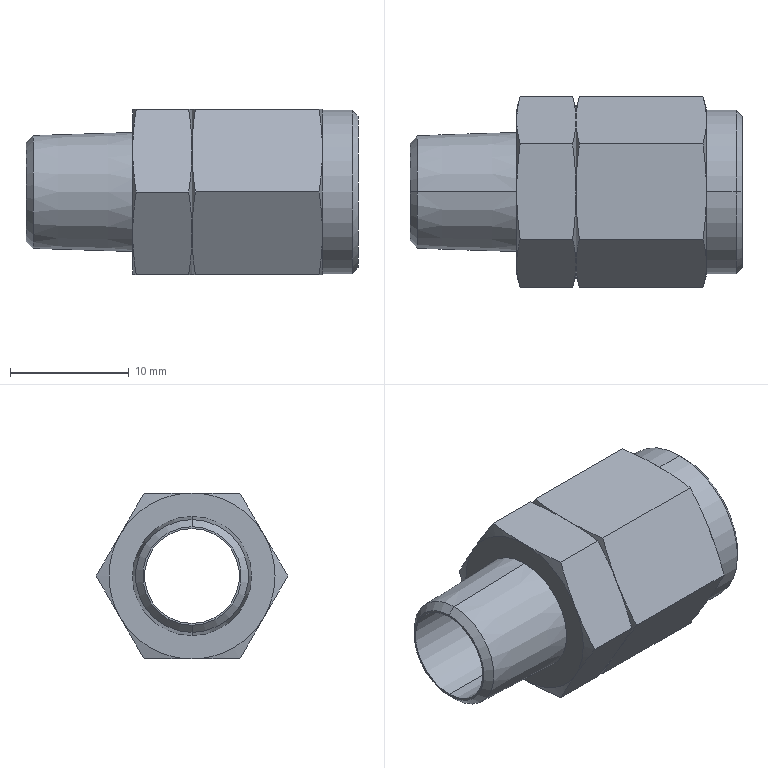Part | STEP file | TJBNC8-1 | 1 solid | 50 faces | box 28 x 16.166 x 14 mm | volume 2415 mm3 | cone 30 | plane 16 | cylinder 4 | commonest cylinder face diameters 8 x2 13.8 x2